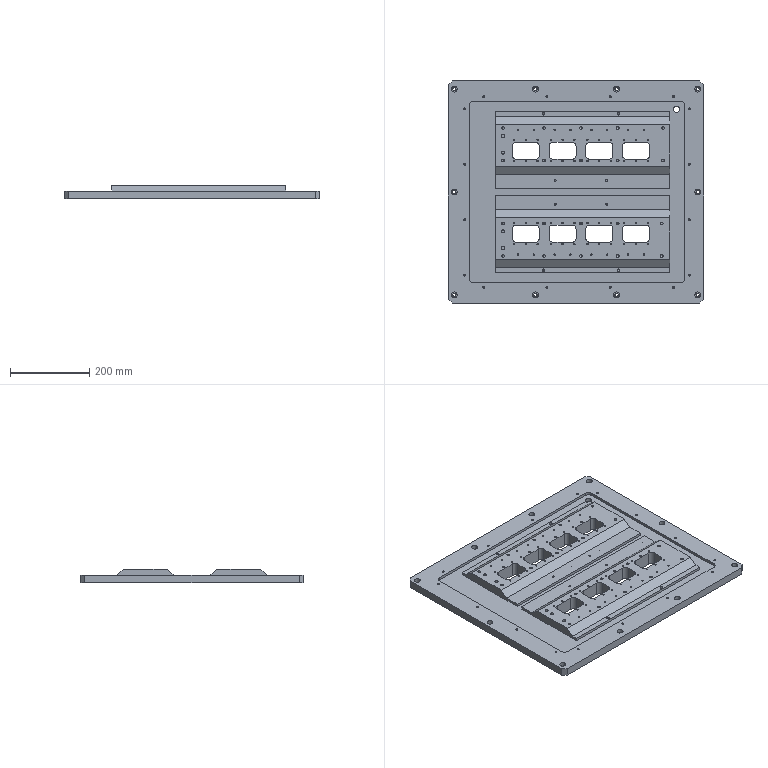Part | SolidWorks | features HoleWzd 10, ICE 3, Chamfer 1, Extrusion 1, Fillet 1 | 1 solid | 677 faces | box 645 x 562 x 35 mm | volume 7508187 mm3 | cylinder 342 | cone 256 | plane 79 | commonest cylinder face diameters 3.3 x128 6.8 x88 5 x40 20 x36 8.4 x20 15 x20